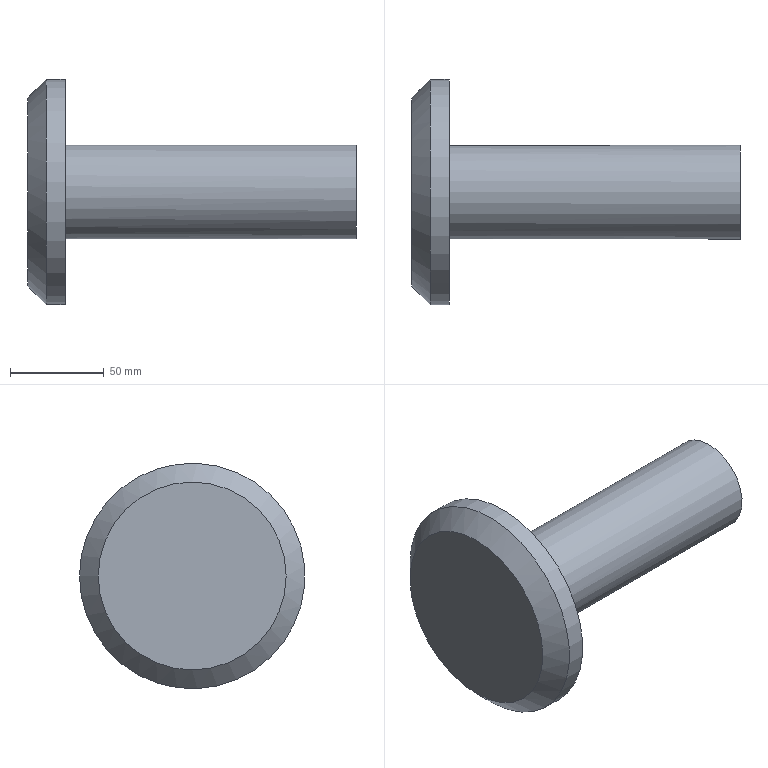Part | NX | features solid 2 | 1 solid | 6 faces | box 175 x 120 x 120 mm | volume 512734 mm3 | plane 3 | cylinder 2 | cone 1 | commonest cylinder face diameters 50 x1 120 x1
STEP:
#1=CARTESIAN_POINT('',(-555.,525.,70.));
#2=VERTEX_POINT('',#1);
#3=CARTESIAN_POINT('',(-555.,525.,45.));
#4=DIRECTION('',(1.,0.,0.));
#5=DIRECTION('',(0.,0.,1.));
#6=AXIS2_PLACEMENT_3D('',#3,#4,#5);
#7=CIRCLE('',#6,25.);
#8=EDGE_CURVE('',#2,#2,#7,.F.);
#9=ORIENTED_EDGE('',*,*,#8,.F.);
#10=EDGE_LOOP('',(#9));
#11=FACE_BOUND('',#10,.T.);
#12=CARTESIAN_POINT('',(-400.,550.,45.));
#13=VERTEX_POINT('',#12);
#14=CARTESIAN_POINT('',(-400.,525.,45.));
#15=DIRECTION('',(1.,0.,0.));
#16=DIRECTION('',(0.,1.,0.));
#17=AXIS2_PLACEMENT_3D('',#14,#15,#16);
#18=CIRCLE('',#17,25.);
#19=EDGE_CURVE('',#13,#13,#18,.T.);
#20=ORIENTED_EDGE('',*,*,#19,.F.);
#21=EDGE_LOOP('',(#20));
#22=FACE_BOUND('',#21,.T.);
#23=CARTESIAN_POINT('',(-555.,525.,45.));
#24=DIRECTION('',(1.,0.,0.));
#25=DIRECTION('',(0.,0.,1.));
#26=AXIS2_PLACEMENT_3D('',#23,#24,#25);
#27=CYLINDRICAL_SURFACE('',#26,25.);
#28=ADVANCED_FACE('',(#11,#22),#27,.T.);
#29=ORIENTED_EDGE('',*,*,#19,.T.);
#30=EDGE_LOOP('',(#29));
#31=FACE_BOUND('',#30,.T.);
#32=CARTESIAN_POINT('',(-400.,525.,45.));
#33=DIRECTION('',(1.,0.,0.));
#34=DIRECTION('',(0.,0.,1.));
#35=AXIS2_PLACEMENT_3D('',#32,#33,#34);
#36=PLANE('',#35);
#37=ADVANCED_FACE('',(#31),#36,.T.);
#38=CARTESIAN_POINT('',(-565.,585.,45.));
#39=VERTEX_POINT('',#38);
#40=CARTESIAN_POINT('',(-565.,525.,45.));
#41=DIRECTION('',(1.,0.,0.));
#42=DIRECTION('',(0.,1.,0.));
#43=AXIS2_PLACEMENT_3D('',#40,#41,#42);
#44=CIRCLE('',#43,60.);
#45=EDGE_CURVE('',#39,#39,#44,.T.);
#46=ORIENTED_EDGE('',*,*,#45,.T.);
#47=EDGE_LOOP('',(#46));
#48=FACE_BOUND('',#47,.T.);
#49=CARTESIAN_POINT('',(-555.,585.,45.));
#50=VERTEX_POINT('',#49);
#51=CARTESIAN_POINT('',(-555.,525.,45.));
#52=DIRECTION('',(1.,0.,0.));
#53=DIRECTION('',(0.,1.,0.));
#54=AXIS2_PLACEMENT_3D('',#51,#52,#53);
#55=CIRCLE('',#54,60.);
#56=EDGE_CURVE('',#50,#50,#55,.T.);
#57=ORIENTED_EDGE('',*,*,#56,.F.);
#58=EDGE_LOOP('',(#57));
#59=FACE_BOUND('',#58,.T.);
#60=CARTESIAN_POINT('',(-565.,525.,45.));
#61=DIRECTION('',(1.,0.,0.));
#62=DIRECTION('',(0.,0.,1.));
#63=AXIS2_PLACEMENT_3D('',#60,#61,#62);
#64=CYLINDRICAL_SURFACE('',#63,60.);
#65=ADVANCED_FACE('',(#48,#59),#64,.T.);
#66=ORIENTED_EDGE('',*,*,#8,.T.);
#67=EDGE_LOOP('',(#66));
#68=FACE_BOUND('',#67,.T.);
#69=ORIENTED_EDGE('',*,*,#56,.T.);
#70=EDGE_LOOP('',(#69));
#71=FACE_BOUND('',#70,.T.);
#72=CARTESIAN_POINT('',(-555.,525.,45.));
#73=DIRECTION('',(1.,0.,0.));
#74=DIRECTION('',(0.,0.,1.));
#75=AXIS2_PLACEMENT_3D('',#72,#73,#74);
#76=PLANE('',#75);
#77=ADVANCED_FACE('',(#68,#71),#76,.T.);
#78=CARTESIAN_POINT('',(-575.,525.,95.));
#79=VERTEX_POINT('',#78);
#80=CARTESIAN_POINT('',(-575.,525.,45.));
#81=DIRECTION('',(1.,0.,0.));
#82=DIRECTION('',(0.,0.,1.));
#83=AXIS2_PLACEMENT_3D('',#80,#81,#82);
#84=CIRCLE('',#83,50.);
#85=EDGE_CURVE('',#79,#79,#84,.T.);
#86=ORIENTED_EDGE('',*,*,#85,.T.);
#87=EDGE_LOOP('',(#86));
#88=FACE_BOUND('',#87,.T.);
#89=ORIENTED_EDGE('',*,*,#45,.F.);
#90=EDGE_LOOP('',(#89));
#91=FACE_BOUND('',#90,.T.);
#92=CARTESIAN_POINT('',(-565.,525.,45.));
#93=DIRECTION('',(1.,0.,0.));
#94=DIRECTION('',(0.,0.,-1.));
#95=AXIS2_PLACEMENT_3D('',#92,#93,#94);
#96=CONICAL_SURFACE('',#95,60.,0.7854);
#97=ADVANCED_FACE('',(#88,#91),#96,.T.);
#98=ORIENTED_EDGE('',*,*,#85,.F.);
#99=EDGE_LOOP('',(#98));
#100=FACE_BOUND('',#99,.T.);
#101=CARTESIAN_POINT('',(-575.,525.,45.));
#102=DIRECTION('',(1.,0.,0.));
#103=DIRECTION('',(0.,0.,1.));
#104=AXIS2_PLACEMENT_3D('',#101,#102,#103);
#105=PLANE('',#104);
#106=ADVANCED_FACE('',(#100),#105,.F.);
#107=CLOSED_SHELL('',(#28,#37,#65,#77,#97,#106));
#108=MANIFOLD_SOLID_BREP('',#107);
#109=(LENGTH_UNIT()NAMED_UNIT(*)SI_UNIT(.MILLI.,.METRE.));
#110=UNCERTAINTY_MEASURE_WITH_UNIT(LENGTH_MEASURE(0.00001),#109,'','');
#111=(NAMED_UNIT(*)PLANE_ANGLE_UNIT()SI_UNIT($,.RADIAN.));
#112=(NAMED_UNIT(*)SI_UNIT($,.STERADIAN.)SOLID_ANGLE_UNIT());
#113=(GEOMETRIC_REPRESENTATION_CONTEXT(3)GLOBAL_UNCERTAINTY_ASSIGNED_CONTEXT((#110))GLOBAL_UNIT_ASSIGNED_CONTEXT((#109,#111,#112))REPRESENTATION_CONTEXT('',''));
#114=ADVANCED_BREP_SHAPE_REPRESENTATION('',(#108),#113);